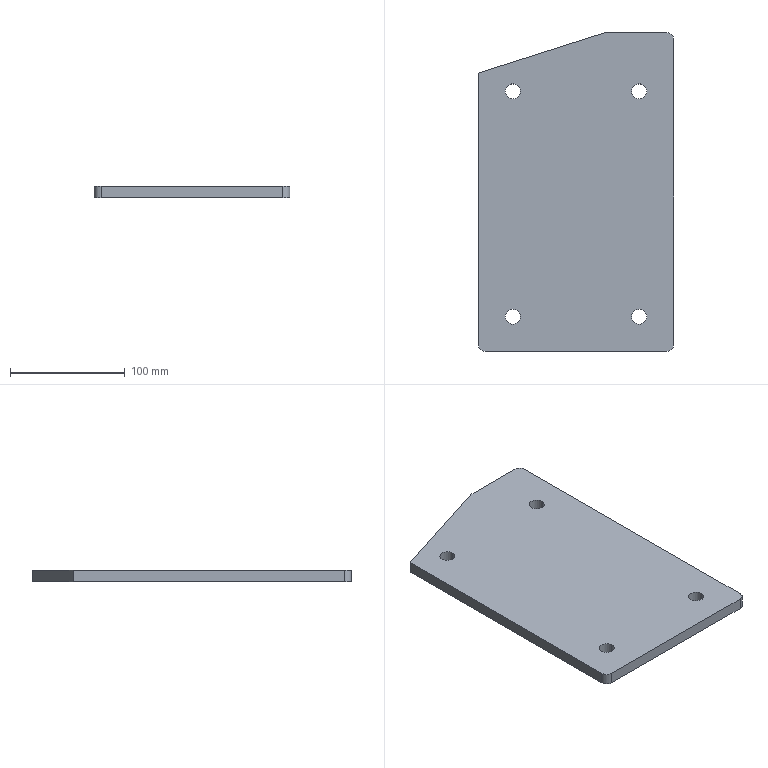Part | SolidWorks | features BaseBody 1 | 1 solid | 18 faces | box 170 x 277 x 10 mm | volume 446109 mm3 | cylinder 11 | plane 7 | commonest cylinder face diameters 13 x8 12 x3
STEP:
#1=CARTESIAN_POINT('',(-61.5,-108.5,0.));
#2=VERTEX_POINT('',#1);
#3=CARTESIAN_POINT('',(-48.5,-108.5,0.));
#4=VERTEX_POINT('',#3);
#5=CARTESIAN_POINT('',(-55.,-108.5,0.));
#6=DIRECTION('',(0.,0.,1.));
#7=DIRECTION('',(1.,0.,0.));
#8=AXIS2_PLACEMENT_3D('',#5,#6,#7);
#9=CIRCLE('',#8,6.5);
#10=EDGE_CURVE('',#2,#4,#9,.T.);
#11=ORIENTED_EDGE('',*,*,#10,.F.);
#12=CARTESIAN_POINT('',(-61.5,-108.5,10.));
#13=VERTEX_POINT('',#12);
#14=CARTESIAN_POINT('',(-61.5,-108.5,0.));
#15=DIRECTION('',(0.,0.,1.));
#16=VECTOR('',#15,1000.);
#17=LINE('',#14,#16);
#18=EDGE_CURVE('',#2,#13,#17,.T.);
#19=ORIENTED_EDGE('',*,*,#18,.T.);
#20=CARTESIAN_POINT('',(-48.5,-108.5,10.));
#21=VERTEX_POINT('',#20);
#22=CARTESIAN_POINT('',(-55.,-108.5,10.));
#23=DIRECTION('',(0.,0.,-1.));
#24=DIRECTION('',(1.,0.,0.));
#25=AXIS2_PLACEMENT_3D('',#22,#23,#24);
#26=CIRCLE('',#25,6.5);
#27=EDGE_CURVE('',#21,#13,#26,.T.);
#28=ORIENTED_EDGE('',*,*,#27,.F.);
#29=CARTESIAN_POINT('',(-48.5,-108.5,0.));
#30=DIRECTION('',(0.,0.,1.));
#31=VECTOR('',#30,1000.);
#32=LINE('',#29,#31);
#33=EDGE_CURVE('',#4,#21,#32,.T.);
#34=ORIENTED_EDGE('',*,*,#33,.F.);
#35=EDGE_LOOP('',(#11,#19,#28,#34));
#36=FACE_OUTER_BOUND('',#35,.T.);
#37=CARTESIAN_POINT('',(-55.,-108.5,0.));
#38=DIRECTION('',(0.,0.,1.));
#39=DIRECTION('',(1.,0.,0.));
#40=AXIS2_PLACEMENT_3D('',#37,#38,#39);
#41=CYLINDRICAL_SURFACE('',#40,6.5);
#42=ADVANCED_FACE('',(#36),#41,.F.);
#43=CARTESIAN_POINT('',(48.5,-108.5,0.));
#44=VERTEX_POINT('',#43);
#45=CARTESIAN_POINT('',(61.5,-108.5,0.));
#46=VERTEX_POINT('',#45);
#47=CARTESIAN_POINT('',(55.,-108.5,0.));
#48=DIRECTION('',(0.,0.,1.));
#49=DIRECTION('',(1.,0.,0.));
#50=AXIS2_PLACEMENT_3D('',#47,#48,#49);
#51=CIRCLE('',#50,6.5);
#52=EDGE_CURVE('',#44,#46,#51,.T.);
#53=ORIENTED_EDGE('',*,*,#52,.F.);
#54=CARTESIAN_POINT('',(48.5,-108.5,10.));
#55=VERTEX_POINT('',#54);
#56=CARTESIAN_POINT('',(48.5,-108.5,0.));
#57=DIRECTION('',(0.,0.,1.));
#58=VECTOR('',#57,1000.);
#59=LINE('',#56,#58);
#60=EDGE_CURVE('',#44,#55,#59,.T.);
#61=ORIENTED_EDGE('',*,*,#60,.T.);
#62=CARTESIAN_POINT('',(61.5,-108.5,10.));
#63=VERTEX_POINT('',#62);
#64=CARTESIAN_POINT('',(55.,-108.5,10.));
#65=DIRECTION('',(0.,0.,-1.));
#66=DIRECTION('',(1.,0.,0.));
#67=AXIS2_PLACEMENT_3D('',#64,#65,#66);
#68=CIRCLE('',#67,6.5);
#69=EDGE_CURVE('',#63,#55,#68,.T.);
#70=ORIENTED_EDGE('',*,*,#69,.F.);
#71=CARTESIAN_POINT('',(61.5,-108.5,0.));
#72=DIRECTION('',(0.,0.,1.));
#73=VECTOR('',#72,1000.);
#74=LINE('',#71,#73);
#75=EDGE_CURVE('',#46,#63,#74,.T.);
#76=ORIENTED_EDGE('',*,*,#75,.F.);
#77=EDGE_LOOP('',(#53,#61,#70,#76));
#78=FACE_OUTER_BOUND('',#77,.T.);
#79=CARTESIAN_POINT('',(55.,-108.5,0.));
#80=DIRECTION('',(0.,0.,1.));
#81=DIRECTION('',(1.,0.,0.));
#82=AXIS2_PLACEMENT_3D('',#79,#80,#81);
#83=CYLINDRICAL_SURFACE('',#82,6.5);
#84=ADVANCED_FACE('',(#78),#83,.F.);
#85=CARTESIAN_POINT('',(48.5,87.5,0.));
#86=VERTEX_POINT('',#85);
#87=CARTESIAN_POINT('',(61.5,87.5,0.));
#88=VERTEX_POINT('',#87);
#89=CARTESIAN_POINT('',(55.,87.5,0.));
#90=DIRECTION('',(0.,0.,1.));
#91=DIRECTION('',(1.,0.,0.));
#92=AXIS2_PLACEMENT_3D('',#89,#90,#91);
#93=CIRCLE('',#92,6.5);
#94=EDGE_CURVE('',#86,#88,#93,.T.);
#95=ORIENTED_EDGE('',*,*,#94,.F.);
#96=CARTESIAN_POINT('',(48.5,87.5,10.));
#97=VERTEX_POINT('',#96);
#98=CARTESIAN_POINT('',(48.5,87.5,0.));
#99=DIRECTION('',(0.,0.,1.));
#100=VECTOR('',#99,1000.);
#101=LINE('',#98,#100);
#102=EDGE_CURVE('',#86,#97,#101,.T.);
#103=ORIENTED_EDGE('',*,*,#102,.T.);
#104=CARTESIAN_POINT('',(61.5,87.5,10.));
#105=VERTEX_POINT('',#104);
#106=CARTESIAN_POINT('',(55.,87.5,10.));
#107=DIRECTION('',(0.,0.,-1.));
#108=DIRECTION('',(1.,0.,0.));
#109=AXIS2_PLACEMENT_3D('',#106,#107,#108);
#110=CIRCLE('',#109,6.5);
#111=EDGE_CURVE('',#105,#97,#110,.T.);
#112=ORIENTED_EDGE('',*,*,#111,.F.);
#113=CARTESIAN_POINT('',(61.5,87.5,0.));
#114=DIRECTION('',(0.,0.,1.));
#115=VECTOR('',#114,1000.);
#116=LINE('',#113,#115);
#117=EDGE_CURVE('',#88,#105,#116,.T.);
#118=ORIENTED_EDGE('',*,*,#117,.F.);
#119=EDGE_LOOP('',(#95,#103,#112,#118));
#120=FACE_OUTER_BOUND('',#119,.T.);
#121=CARTESIAN_POINT('',(55.,87.5,0.));
#122=DIRECTION('',(0.,0.,1.));
#123=DIRECTION('',(1.,0.,0.));
#124=AXIS2_PLACEMENT_3D('',#121,#122,#123);
#125=CYLINDRICAL_SURFACE('',#124,6.5);
#126=ADVANCED_FACE('',(#120),#125,.F.);
#127=CARTESIAN_POINT('',(-61.5,87.5,0.));
#128=VERTEX_POINT('',#127);
#129=CARTESIAN_POINT('',(-48.5,87.5,0.));
#130=VERTEX_POINT('',#129);
#131=CARTESIAN_POINT('',(-55.,87.5,0.));
#132=DIRECTION('',(0.,0.,1.));
#133=DIRECTION('',(1.,0.,0.));
#134=AXIS2_PLACEMENT_3D('',#131,#132,#133);
#135=CIRCLE('',#134,6.5);
#136=EDGE_CURVE('',#128,#130,#135,.T.);
#137=ORIENTED_EDGE('',*,*,#136,.F.);
#138=CARTESIAN_POINT('',(-61.5,87.5,10.));
#139=VERTEX_POINT('',#138);
#140=CARTESIAN_POINT('',(-61.5,87.5,0.));
#141=DIRECTION('',(0.,0.,1.));
#142=VECTOR('',#141,1000.);
#143=LINE('',#140,#142);
#144=EDGE_CURVE('',#128,#139,#143,.T.);
#145=ORIENTED_EDGE('',*,*,#144,.T.);
#146=CARTESIAN_POINT('',(-48.5,87.5,10.));
#147=VERTEX_POINT('',#146);
#148=CARTESIAN_POINT('',(-55.,87.5,10.));
#149=DIRECTION('',(0.,0.,-1.));
#150=DIRECTION('',(1.,0.,0.));
#151=AXIS2_PLACEMENT_3D('',#148,#149,#150);
#152=CIRCLE('',#151,6.5);
#153=EDGE_CURVE('',#147,#139,#152,.T.);
#154=ORIENTED_EDGE('',*,*,#153,.F.);
#155=CARTESIAN_POINT('',(-48.5,87.5,0.));
#156=DIRECTION('',(0.,0.,1.));
#157=VECTOR('',#156,1000.);
#158=LINE('',#155,#157);
#159=EDGE_CURVE('',#130,#147,#158,.T.);
#160=ORIENTED_EDGE('',*,*,#159,.F.);
#161=EDGE_LOOP('',(#137,#145,#154,#160));
#162=FACE_OUTER_BOUND('',#161,.T.);
#163=CARTESIAN_POINT('',(-55.,87.5,0.));
#164=DIRECTION('',(0.,0.,1.));
#165=DIRECTION('',(1.,0.,0.));
#166=AXIS2_PLACEMENT_3D('',#163,#164,#165);
#167=CYLINDRICAL_SURFACE('',#166,6.5);
#168=ADVANCED_FACE('',(#162),#167,.F.);
#169=ORIENTED_EDGE('',*,*,#27,.T.);
#170=CARTESIAN_POINT('',(-55.,-108.5,10.));
#171=DIRECTION('',(0.,0.,-1.));
#172=DIRECTION('',(1.,0.,0.));
#173=AXIS2_PLACEMENT_3D('',#170,#171,#172);
#174=CIRCLE('',#173,6.5);
#175=EDGE_CURVE('',#13,#21,#174,.T.);
#176=ORIENTED_EDGE('',*,*,#175,.T.);
#177=EDGE_LOOP('',(#169,#176));
#178=FACE_BOUND('',#177,.T.);
#179=ORIENTED_EDGE('',*,*,#69,.T.);
#180=CARTESIAN_POINT('',(55.,-108.5,10.));
#181=DIRECTION('',(0.,0.,-1.));
#182=DIRECTION('',(1.,0.,0.));
#183=AXIS2_PLACEMENT_3D('',#180,#181,#182);
#184=CIRCLE('',#183,6.5);
#185=EDGE_CURVE('',#55,#63,#184,.T.);
#186=ORIENTED_EDGE('',*,*,#185,.T.);
#187=EDGE_LOOP('',(#179,#186));
#188=FACE_BOUND('',#187,.T.);
#189=ORIENTED_EDGE('',*,*,#111,.T.);
#190=CARTESIAN_POINT('',(55.,87.5,10.));
#191=DIRECTION('',(0.,0.,-1.));
#192=DIRECTION('',(1.,0.,0.));
#193=AXIS2_PLACEMENT_3D('',#190,#191,#192);
#194=CIRCLE('',#193,6.5);
#195=EDGE_CURVE('',#97,#105,#194,.T.);
#196=ORIENTED_EDGE('',*,*,#195,.T.);
#197=EDGE_LOOP('',(#189,#196));
#198=FACE_BOUND('',#197,.T.);
#199=ORIENTED_EDGE('',*,*,#153,.T.);
#200=CARTESIAN_POINT('',(-55.,87.5,10.));
#201=DIRECTION('',(0.,0.,-1.));
#202=DIRECTION('',(1.,0.,0.));
#203=AXIS2_PLACEMENT_3D('',#200,#201,#202);
#204=CIRCLE('',#203,6.5);
#205=EDGE_CURVE('',#139,#147,#204,.T.);
#206=ORIENTED_EDGE('',*,*,#205,.T.);
#207=EDGE_LOOP('',(#199,#206));
#208=FACE_BOUND('',#207,.T.);
#209=CARTESIAN_POINT('',(85.,132.5,10.));
#210=VERTEX_POINT('',#209);
#211=CARTESIAN_POINT('',(79.,138.5,10.));
#212=VERTEX_POINT('',#211);
#213=CARTESIAN_POINT('',(79.,132.5,10.));
#214=DIRECTION('',(0.,0.,1.));
#215=DIRECTION('',(1.,0.,0.));
#216=AXIS2_PLACEMENT_3D('',#213,#214,#215);
#217=CIRCLE('',#216,6.);
#218=EDGE_CURVE('',#210,#212,#217,.T.);
#219=ORIENTED_EDGE('',*,*,#218,.T.);
#220=CARTESIAN_POINT('',(25.,138.5,10.));
#221=VERTEX_POINT('',#220);
#222=CARTESIAN_POINT('',(0.,138.5,10.));
#223=DIRECTION('',(-1.,0.,0.));
#224=VECTOR('',#223,1000.);
#225=LINE('',#222,#224);
#226=EDGE_CURVE('',#212,#221,#225,.T.);
#227=ORIENTED_EDGE('',*,*,#226,.T.);
#228=CARTESIAN_POINT('',(-85.,103.5,10.));
#229=VERTEX_POINT('',#228);
#230=CARTESIAN_POINT('',(25.,138.5,10.));
#231=DIRECTION('',(-0.9529,-0.3032,0.));
#232=VECTOR('',#231,1000.);
#233=LINE('',#230,#232);
#234=EDGE_CURVE('',#221,#229,#233,.T.);
#235=ORIENTED_EDGE('',*,*,#234,.T.);
#236=CARTESIAN_POINT('',(-85.,-132.5,10.));
#237=VERTEX_POINT('',#236);
#238=CARTESIAN_POINT('',(-85.,0.,10.));
#239=DIRECTION('',(0.,-1.,0.));
#240=VECTOR('',#239,1000.);
#241=LINE('',#238,#240);
#242=EDGE_CURVE('',#229,#237,#241,.T.);
#243=ORIENTED_EDGE('',*,*,#242,.T.);
#244=CARTESIAN_POINT('',(-79.,-138.5,10.));
#245=VERTEX_POINT('',#244);
#246=CARTESIAN_POINT('',(-79.,-132.5,10.));
#247=DIRECTION('',(0.,0.,1.));
#248=DIRECTION('',(1.,0.,0.));
#249=AXIS2_PLACEMENT_3D('',#246,#247,#248);
#250=CIRCLE('',#249,6.);
#251=EDGE_CURVE('',#237,#245,#250,.T.);
#252=ORIENTED_EDGE('',*,*,#251,.T.);
#253=CARTESIAN_POINT('',(79.,-138.5,10.));
#254=VERTEX_POINT('',#253);
#255=CARTESIAN_POINT('',(0.,-138.5,10.));
#256=DIRECTION('',(1.,0.,0.));
#257=VECTOR('',#256,1000.);
#258=LINE('',#255,#257);
#259=EDGE_CURVE('',#245,#254,#258,.T.);
#260=ORIENTED_EDGE('',*,*,#259,.T.);
#261=CARTESIAN_POINT('',(85.,-132.5,10.));
#262=VERTEX_POINT('',#261);
#263=CARTESIAN_POINT('',(79.,-132.5,10.));
#264=DIRECTION('',(0.,0.,1.));
#265=DIRECTION('',(1.,0.,0.));
#266=AXIS2_PLACEMENT_3D('',#263,#264,#265);
#267=CIRCLE('',#266,6.);
#268=EDGE_CURVE('',#254,#262,#267,.T.);
#269=ORIENTED_EDGE('',*,*,#268,.T.);
#270=CARTESIAN_POINT('',(85.,0.,10.));
#271=DIRECTION('',(0.,1.,0.));
#272=VECTOR('',#271,1000.);
#273=LINE('',#270,#272);
#274=EDGE_CURVE('',#262,#210,#273,.T.);
#275=ORIENTED_EDGE('',*,*,#274,.T.);
#276=EDGE_LOOP('',(#219,#227,#235,#243,#252,#260,#269,#275));
#277=FACE_OUTER_BOUND('',#276,.T.);
#278=CARTESIAN_POINT('',(0.,0.,10.));
#279=DIRECTION('',(0.,0.,1.));
#280=DIRECTION('',(1.,0.,0.));
#281=AXIS2_PLACEMENT_3D('',#278,#279,#280);
#282=PLANE('',#281);
#283=ADVANCED_FACE('',(#178,#188,#198,#208,#277),#282,.T.);
#284=ORIENTED_EDGE('',*,*,#18,.F.);
#285=CARTESIAN_POINT('',(-55.,-108.5,0.));
#286=DIRECTION('',(0.,0.,1.));
#287=DIRECTION('',(1.,0.,0.));
#288=AXIS2_PLACEMENT_3D('',#285,#286,#287);
#289=CIRCLE('',#288,6.5);
#290=EDGE_CURVE('',#4,#2,#289,.T.);
#291=ORIENTED_EDGE('',*,*,#290,.F.);
#292=ORIENTED_EDGE('',*,*,#33,.T.);
#293=ORIENTED_EDGE('',*,*,#175,.F.);
#294=EDGE_LOOP('',(#284,#291,#292,#293));
#295=FACE_OUTER_BOUND('',#294,.T.);
#296=CARTESIAN_POINT('',(-55.,-108.5,0.));
#297=DIRECTION('',(0.,0.,1.));
#298=DIRECTION('',(1.,0.,0.));
#299=AXIS2_PLACEMENT_3D('',#296,#297,#298);
#300=CYLINDRICAL_SURFACE('',#299,6.5);
#301=ADVANCED_FACE('',(#295),#300,.F.);
#302=ORIENTED_EDGE('',*,*,#60,.F.);
#303=CARTESIAN_POINT('',(55.,-108.5,0.));
#304=DIRECTION('',(0.,0.,1.));
#305=DIRECTION('',(1.,0.,0.));
#306=AXIS2_PLACEMENT_3D('',#303,#304,#305);
#307=CIRCLE('',#306,6.5);
#308=EDGE_CURVE('',#46,#44,#307,.T.);
#309=ORIENTED_EDGE('',*,*,#308,.F.);
#310=ORIENTED_EDGE('',*,*,#75,.T.);
#311=ORIENTED_EDGE('',*,*,#185,.F.);
#312=EDGE_LOOP('',(#302,#309,#310,#311));
#313=FACE_OUTER_BOUND('',#312,.T.);
#314=CARTESIAN_POINT('',(55.,-108.5,0.));
#315=DIRECTION('',(0.,0.,1.));
#316=DIRECTION('',(1.,0.,0.));
#317=AXIS2_PLACEMENT_3D('',#314,#315,#316);
#318=CYLINDRICAL_SURFACE('',#317,6.5);
#319=ADVANCED_FACE('',(#313),#318,.F.);
#320=ORIENTED_EDGE('',*,*,#102,.F.);
#321=CARTESIAN_POINT('',(55.,87.5,0.));
#322=DIRECTION('',(0.,0.,1.));
#323=DIRECTION('',(1.,0.,0.));
#324=AXIS2_PLACEMENT_3D('',#321,#322,#323);
#325=CIRCLE('',#324,6.5);
#326=EDGE_CURVE('',#88,#86,#325,.T.);
#327=ORIENTED_EDGE('',*,*,#326,.F.);
#328=ORIENTED_EDGE('',*,*,#117,.T.);
#329=ORIENTED_EDGE('',*,*,#195,.F.);
#330=EDGE_LOOP('',(#320,#327,#328,#329));
#331=FACE_OUTER_BOUND('',#330,.T.);
#332=CARTESIAN_POINT('',(55.,87.5,0.));
#333=DIRECTION('',(0.,0.,1.));
#334=DIRECTION('',(1.,0.,0.));
#335=AXIS2_PLACEMENT_3D('',#332,#333,#334);
#336=CYLINDRICAL_SURFACE('',#335,6.5);
#337=ADVANCED_FACE('',(#331),#336,.F.);
#338=ORIENTED_EDGE('',*,*,#144,.F.);
#339=CARTESIAN_POINT('',(-55.,87.5,0.));
#340=DIRECTION('',(0.,0.,1.));
#341=DIRECTION('',(1.,0.,0.));
#342=AXIS2_PLACEMENT_3D('',#339,#340,#341);
#343=CIRCLE('',#342,6.5);
#344=EDGE_CURVE('',#130,#128,#343,.T.);
#345=ORIENTED_EDGE('',*,*,#344,.F.);
#346=ORIENTED_EDGE('',*,*,#159,.T.);
#347=ORIENTED_EDGE('',*,*,#205,.F.);
#348=EDGE_LOOP('',(#338,#345,#346,#347));
#349=FACE_OUTER_BOUND('',#348,.T.);
#350=CARTESIAN_POINT('',(-55.,87.5,0.));
#351=DIRECTION('',(0.,0.,1.));
#352=DIRECTION('',(1.,0.,0.));
#353=AXIS2_PLACEMENT_3D('',#350,#351,#352);
#354=CYLINDRICAL_SURFACE('',#353,6.5);
#355=ADVANCED_FACE('',(#349),#354,.F.);
#356=CARTESIAN_POINT('',(79.,138.5,0.));
#357=VERTEX_POINT('',#356);
#358=CARTESIAN_POINT('',(79.,138.5,0.));
#359=DIRECTION('',(0.,0.,-1.));
#360=VECTOR('',#359,1000.);
#361=LINE('',#358,#360);
#362=EDGE_CURVE('',#212,#357,#361,.T.);
#363=ORIENTED_EDGE('',*,*,#362,.T.);
#364=CARTESIAN_POINT('',(25.,138.5,0.));
#365=VERTEX_POINT('',#364);
#366=CARTESIAN_POINT('',(-85.,138.5,0.));
#367=DIRECTION('',(-1.,0.,0.));
#368=VECTOR('',#367,1000.);
#369=LINE('',#366,#368);
#370=EDGE_CURVE('',#357,#365,#369,.T.);
#371=ORIENTED_EDGE('',*,*,#370,.T.);
#372=CARTESIAN_POINT('',(25.,138.5,0.));
#373=DIRECTION('',(0.,0.,1.));
#374=VECTOR('',#373,1000.);
#375=LINE('',#372,#374);
#376=EDGE_CURVE('',#365,#221,#375,.T.);
#377=ORIENTED_EDGE('',*,*,#376,.T.);
#378=ORIENTED_EDGE('',*,*,#226,.F.);
#379=EDGE_LOOP('',(#363,#371,#377,#378));
#380=FACE_OUTER_BOUND('',#379,.T.);
#381=CARTESIAN_POINT('',(-85.,138.5,0.));
#382=DIRECTION('',(0.,1.,0.));
#383=DIRECTION('',(-1.,0.,0.));
#384=AXIS2_PLACEMENT_3D('',#381,#382,#383);
#385=PLANE('',#384);
#386=ADVANCED_FACE('',(#380),#385,.T.);
#387=CARTESIAN_POINT('',(85.,132.5,0.));
#388=VERTEX_POINT('',#387);
#389=CARTESIAN_POINT('',(79.,132.5,0.));
#390=DIRECTION('',(0.,0.,1.));
#391=DIRECTION('',(1.,0.,0.));
#392=AXIS2_PLACEMENT_3D('',#389,#390,#391);
#393=CIRCLE('',#392,6.);
#394=EDGE_CURVE('',#388,#357,#393,.T.);
#395=ORIENTED_EDGE('',*,*,#394,.T.);
#396=ORIENTED_EDGE('',*,*,#362,.F.);
#397=ORIENTED_EDGE('',*,*,#218,.F.);
#398=CARTESIAN_POINT('',(85.,132.5,0.));
#399=DIRECTION('',(0.,0.,-1.));
#400=VECTOR('',#399,1000.);
#401=LINE('',#398,#400);
#402=EDGE_CURVE('',#210,#388,#401,.T.);
#403=ORIENTED_EDGE('',*,*,#402,.T.);
#404=EDGE_LOOP('',(#395,#396,#397,#403));
#405=FACE_OUTER_BOUND('',#404,.T.);
#406=CARTESIAN_POINT('',(79.,132.5,0.));
#407=DIRECTION('',(0.,0.,1.));
#408=DIRECTION('',(1.,0.,0.));
#409=AXIS2_PLACEMENT_3D('',#406,#407,#408);
#410=CYLINDRICAL_SURFACE('',#409,6.);
#411=ADVANCED_FACE('',(#405),#410,.T.);
#412=CARTESIAN_POINT('',(85.,-132.5,0.));
#413=VERTEX_POINT('',#412);
#414=CARTESIAN_POINT('',(85.,-132.5,0.));
#415=DIRECTION('',(0.,0.,-1.));
#416=VECTOR('',#415,1000.);
#417=LINE('',#414,#416);
#418=EDGE_CURVE('',#262,#413,#417,.T.);
#419=ORIENTED_EDGE('',*,*,#418,.T.);
#420=CARTESIAN_POINT('',(85.,138.5,0.));
#421=DIRECTION('',(0.,1.,0.));
#422=VECTOR('',#421,1000.);
#423=LINE('',#420,#422);
#424=EDGE_CURVE('',#413,#388,#423,.T.);
#425=ORIENTED_EDGE('',*,*,#424,.T.);
#426=ORIENTED_EDGE('',*,*,#402,.F.);
#427=ORIENTED_EDGE('',*,*,#274,.F.);
#428=EDGE_LOOP('',(#419,#425,#426,#427));
#429=FACE_OUTER_BOUND('',#428,.T.);
#430=CARTESIAN_POINT('',(85.,138.5,0.));
#431=DIRECTION('',(1.,0.,0.));
#432=DIRECTION('',(0.,1.,0.));
#433=AXIS2_PLACEMENT_3D('',#430,#431,#432);
#434=PLANE('',#433);
#435=ADVANCED_FACE('',(#429),#434,.T.);
#436=CARTESIAN_POINT('',(79.,-138.5,0.));
#437=VERTEX_POINT('',#436);
#438=CARTESIAN_POINT('',(79.,-132.5,0.));
#439=DIRECTION('',(0.,0.,1.));
#440=DIRECTION('',(1.,0.,0.));
#441=AXIS2_PLACEMENT_3D('',#438,#439,#440);
#442=CIRCLE('',#441,6.);
#443=EDGE_CURVE('',#437,#413,#442,.T.);
#444=ORIENTED_EDGE('',*,*,#443,.T.);
#445=ORIENTED_EDGE('',*,*,#418,.F.);
#446=ORIENTED_EDGE('',*,*,#268,.F.);
#447=CARTESIAN_POINT('',(79.,-138.5,0.));
#448=DIRECTION('',(0.,0.,-1.));
#449=VECTOR('',#448,1000.);
#450=LINE('',#447,#449);
#451=EDGE_CURVE('',#254,#437,#450,.T.);
#452=ORIENTED_EDGE('',*,*,#451,.T.);
#453=EDGE_LOOP('',(#444,#445,#446,#452));
#454=FACE_OUTER_BOUND('',#453,.T.);
#455=CARTESIAN_POINT('',(79.,-132.5,0.));
#456=DIRECTION('',(0.,0.,1.));
#457=DIRECTION('',(1.,0.,0.));
#458=AXIS2_PLACEMENT_3D('',#455,#456,#457);
#459=CYLINDRICAL_SURFACE('',#458,6.);
#460=ADVANCED_FACE('',(#454),#459,.T.);
#461=CARTESIAN_POINT('',(-79.,-138.5,0.));
#462=VERTEX_POINT('',#461);
#463=CARTESIAN_POINT('',(-79.,-138.5,0.));
#464=DIRECTION('',(0.,0.,-1.));
#465=VECTOR('',#464,1000.);
#466=LINE('',#463,#465);
#467=EDGE_CURVE('',#245,#462,#466,.T.);
#468=ORIENTED_EDGE('',*,*,#467,.T.);
#469=CARTESIAN_POINT('',(85.,-138.5,0.));
#470=DIRECTION('',(1.,0.,0.));
#471=VECTOR('',#470,1000.);
#472=LINE('',#469,#471);
#473=EDGE_CURVE('',#462,#437,#472,.T.);
#474=ORIENTED_EDGE('',*,*,#473,.T.);
#475=ORIENTED_EDGE('',*,*,#451,.F.);
#476=ORIENTED_EDGE('',*,*,#259,.F.);
#477=EDGE_LOOP('',(#468,#474,#475,#476));
#478=FACE_OUTER_BOUND('',#477,.T.);
#479=CARTESIAN_POINT('',(85.,-138.5,0.));
#480=DIRECTION('',(0.,-1.,0.));
#481=DIRECTION('',(1.,0.,0.));
#482=AXIS2_PLACEMENT_3D('',#479,#480,#481);
#483=PLANE('',#482);
#484=ADVANCED_FACE('',(#478),#483,.T.);
#485=CARTESIAN_POINT('',(-85.,-132.5,0.));
#486=VERTEX_POINT('',#485);
#487=CARTESIAN_POINT('',(-79.,-132.5,0.));
#488=DIRECTION('',(0.,0.,1.));
#489=DIRECTION('',(1.,0.,0.));
#490=AXIS2_PLACEMENT_3D('',#487,#488,#489);
#491=CIRCLE('',#490,6.);
#492=EDGE_CURVE('',#486,#462,#491,.T.);
#493=ORIENTED_EDGE('',*,*,#492,.T.);
#494=ORIENTED_EDGE('',*,*,#467,.F.);
#495=ORIENTED_EDGE('',*,*,#251,.F.);
#496=CARTESIAN_POINT('',(-85.,-132.5,0.));
#497=DIRECTION('',(0.,0.,-1.));
#498=VECTOR('',#497,1000.);
#499=LINE('',#496,#498);
#500=EDGE_CURVE('',#237,#486,#499,.T.);
#501=ORIENTED_EDGE('',*,*,#500,.T.);
#502=EDGE_LOOP('',(#493,#494,#495,#501));
#503=FACE_OUTER_BOUND('',#502,.T.);
#504=CARTESIAN_POINT('',(-79.,-132.5,0.));
#505=DIRECTION('',(0.,0.,1.));
#506=DIRECTION('',(1.,0.,0.));
#507=AXIS2_PLACEMENT_3D('',#504,#505,#506);
#508=CYLINDRICAL_SURFACE('',#507,6.);
#509=ADVANCED_FACE('',(#503),#508,.T.);
#510=ORIENTED_EDGE('',*,*,#500,.F.);
#511=ORIENTED_EDGE('',*,*,#242,.F.);
#512=CARTESIAN_POINT('',(-85.,103.5,0.));
#513=VERTEX_POINT('',#512);
#514=CARTESIAN_POINT('',(-85.,103.5,0.));
#515=DIRECTION('',(0.,0.,-1.));
#516=VECTOR('',#515,1000.);
#517=LINE('',#514,#516);
#518=EDGE_CURVE('',#229,#513,#517,.T.);
#519=ORIENTED_EDGE('',*,*,#518,.T.);
#520=CARTESIAN_POINT('',(-85.,-138.5,0.));
#521=DIRECTION('',(0.,-1.,0.));
#522=VECTOR('',#521,1000.);
#523=LINE('',#520,#522);
#524=EDGE_CURVE('',#513,#486,#523,.T.);
#525=ORIENTED_EDGE('',*,*,#524,.T.);
#526=EDGE_LOOP('',(#510,#511,#519,#525));
#527=FACE_OUTER_BOUND('',#526,.T.);
#528=CARTESIAN_POINT('',(-85.,-138.5,0.));
#529=DIRECTION('',(-1.,0.,0.));
#530=DIRECTION('',(0.,-1.,0.));
#531=AXIS2_PLACEMENT_3D('',#528,#529,#530);
#532=PLANE('',#531);
#533=ADVANCED_FACE('',(#527),#532,.T.);
#534=ORIENTED_EDGE('',*,*,#518,.F.);
#535=ORIENTED_EDGE('',*,*,#234,.F.);
#536=ORIENTED_EDGE('',*,*,#376,.F.);
#537=CARTESIAN_POINT('',(-85.,103.5,0.));
#538=DIRECTION('',(0.9529,0.3032,0.));
#539=VECTOR('',#538,1000.);
#540=LINE('',#537,#539);
#541=EDGE_CURVE('',#513,#365,#540,.T.);
#542=ORIENTED_EDGE('',*,*,#541,.F.);
#543=EDGE_LOOP('',(#534,#535,#536,#542));
#544=FACE_OUTER_BOUND('',#543,.T.);
#545=CARTESIAN_POINT('',(-85.,103.5,0.));
#546=DIRECTION('',(0.3032,-0.9529,0.));
#547=DIRECTION('',(0.9529,0.3032,0.));
#548=AXIS2_PLACEMENT_3D('',#545,#546,#547);
#549=PLANE('',#548);
#550=ADVANCED_FACE('',(#544),#549,.F.);
#551=ORIENTED_EDGE('',*,*,#344,.T.);
#552=ORIENTED_EDGE('',*,*,#136,.T.);
#553=EDGE_LOOP('',(#551,#552));
#554=FACE_BOUND('',#553,.T.);
#555=ORIENTED_EDGE('',*,*,#326,.T.);
#556=ORIENTED_EDGE('',*,*,#94,.T.);
#557=EDGE_LOOP('',(#555,#556));
#558=FACE_BOUND('',#557,.T.);
#559=ORIENTED_EDGE('',*,*,#308,.T.);
#560=ORIENTED_EDGE('',*,*,#52,.T.);
#561=EDGE_LOOP('',(#559,#560));
#562=FACE_BOUND('',#561,.T.);
#563=ORIENTED_EDGE('',*,*,#290,.T.);
#564=ORIENTED_EDGE('',*,*,#10,.T.);
#565=EDGE_LOOP('',(#563,#564));
#566=FACE_BOUND('',#565,.T.);
#567=ORIENTED_EDGE('',*,*,#370,.F.);
#568=ORIENTED_EDGE('',*,*,#394,.F.);
#569=ORIENTED_EDGE('',*,*,#424,.F.);
#570=ORIENTED_EDGE('',*,*,#443,.F.);
#571=ORIENTED_EDGE('',*,*,#473,.F.);
#572=ORIENTED_EDGE('',*,*,#492,.F.);
#573=ORIENTED_EDGE('',*,*,#524,.F.);
#574=ORIENTED_EDGE('',*,*,#541,.T.);
#575=EDGE_LOOP('',(#567,#568,#569,#570,#571,#572,#573,#574));
#576=FACE_OUTER_BOUND('',#575,.T.);
#577=CARTESIAN_POINT('',(0.,0.,0.));
#578=DIRECTION('',(0.,0.,1.));
#579=DIRECTION('',(1.,0.,0.));
#580=AXIS2_PLACEMENT_3D('',#577,#578,#579);
#581=PLANE('',#580);
#582=ADVANCED_FACE('',(#554,#558,#562,#566,#576),#581,.F.);
#583=CLOSED_SHELL('',(#42,#84,#126,#168,#283,#301,#319,#337,#355,#386,#411,#435,#460,#484,#509,#533,#550,#582));
#584=MANIFOLD_SOLID_BREP('',#583);
#585=CARTESIAN_POINT('',(0.,0.,0.));
#586=DIRECTION('',(0.,0.,1.));
#587=DIRECTION('',(1.,0.,0.));
#588=AXIS2_PLACEMENT_3D('',#585,#586,#587);
#589=(LENGTH_UNIT()NAMED_UNIT(*)SI_UNIT(.MILLI.,.METRE.));
#590=UNCERTAINTY_MEASURE_WITH_UNIT(LENGTH_MEASURE(0.00001),#589,'','');
#591=(NAMED_UNIT(*)PLANE_ANGLE_UNIT()SI_UNIT($,.RADIAN.));
#592=(NAMED_UNIT(*)SI_UNIT($,.STERADIAN.)SOLID_ANGLE_UNIT());
#593=(GEOMETRIC_REPRESENTATION_CONTEXT(3)GLOBAL_UNCERTAINTY_ASSIGNED_CONTEXT((#590))GLOBAL_UNIT_ASSIGNED_CONTEXT((#589,#591,#592))REPRESENTATION_CONTEXT('',''));
#594=ADVANCED_BREP_SHAPE_REPRESENTATION('',(#584,#588),#593);